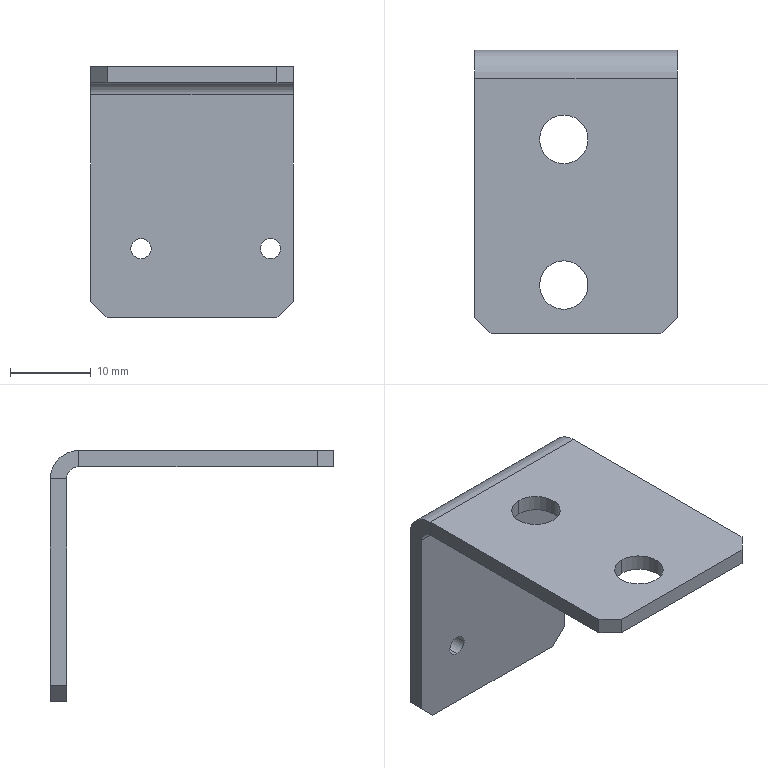Part | STEP file | 227H056375 Sensor BKT_Default | 1 solid | 26 faces | box 25 x 35 x 31 mm | volume 2998 mm3 | plane 16 | cylinder 10 | commonest cylinder face diameters 2.5 x4 6 x4 3 x1 7 x1